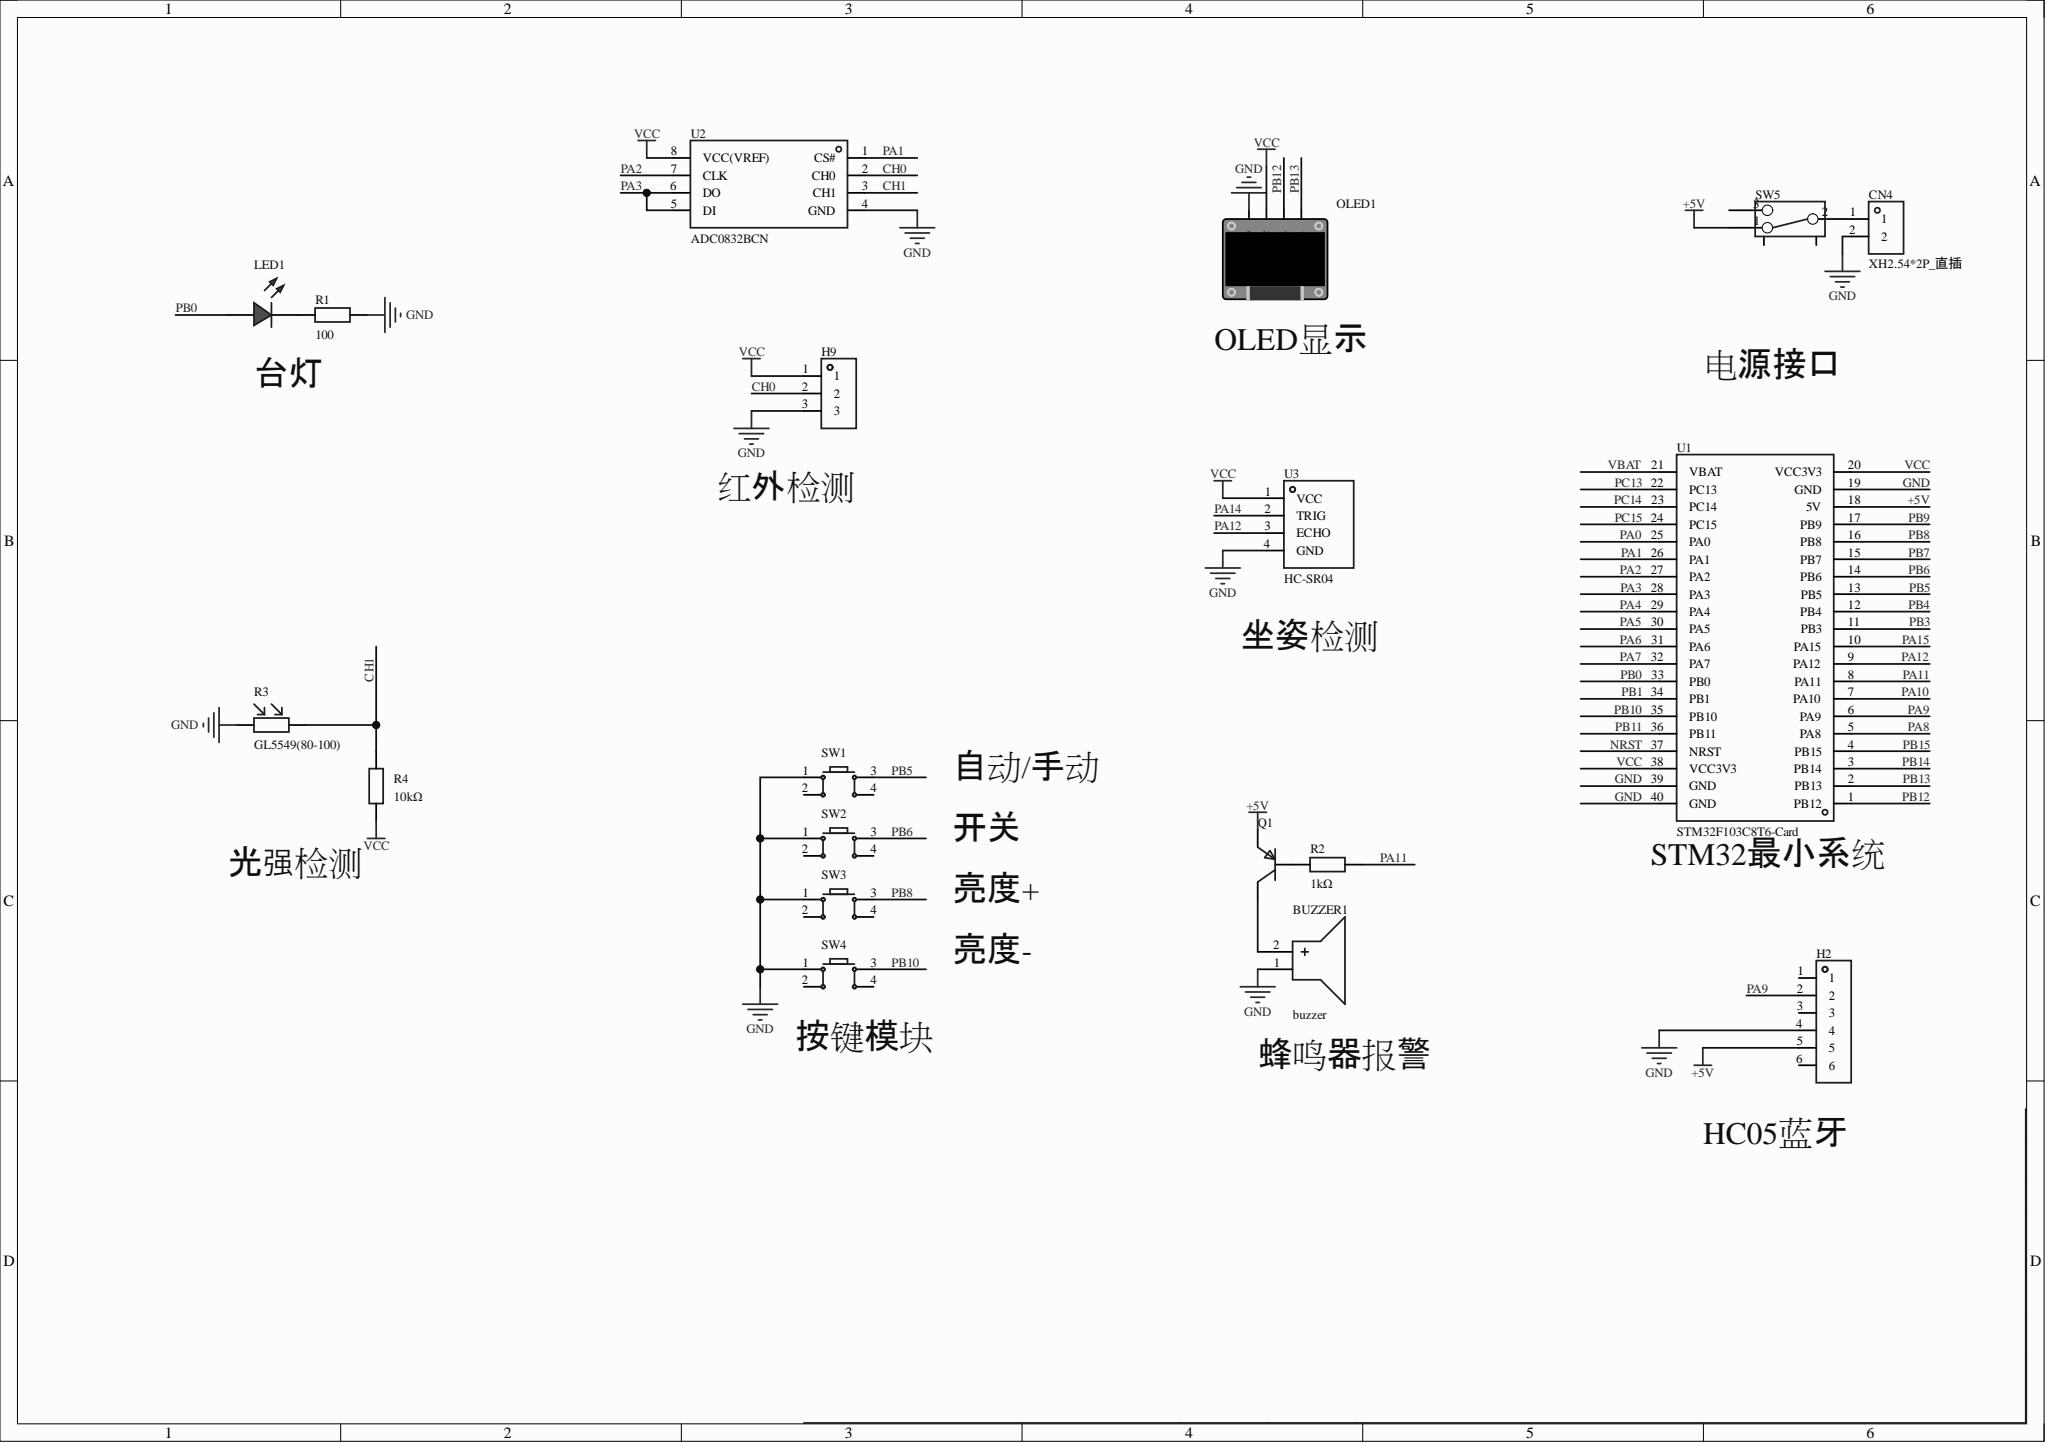Circuit board | Altium Designer | 19 parts | 22 nets
Bill of materials:
Comment,Description,Designator,Footprint,LibRef,Quantity
"buzzer","","BUZZER1","BUZ-TH_BD12.0-P6.00-D0.9-RD","buzzer","1"
"XH2.54*2P_直插","","CN4","CONN-TH_2P-P2.50-XH2.54-2P","XH2.54*2P_直插","1"
"","","H2","HDR-TH_6P-P2.54-V-F","HDR-F_2.54_1x6P","1"
"","","H9","HDR-TH_3P-P2.54-V-F","HDR-F_2.54_1x3P","1"
"","","LED1","LED_TH-3mm","LED_TH-R_3mm","1"
"","","OLED1","0.96OLED_4P","0.96OLED模块_4P","1"
"","","Q1","S8550P_TO-92","S8550_TO_PNP","1"
"100","","R1","Res_1/8W","Res_AXIAL-1/8W","1"
"1kΩ","","R2","Res_1/8W","Res_AXIAL-1/8W","1"
"GL5549(80-100)","","R3","RES-TH_L5.1-W4.3-P3.40-D0.5","GL5549(80-100)","1"
"10kΩ","","R4","Res_1/8W","Res_AXIAL-1/8W","1"
"","","SW1, SW2, SW3, SW4","SW-TH_4P-L6.0-W6.0-P4.50-LS6.5","Key_TH_6x6x6","4"
"","","SW5","拨动开关","拨动开关_正","1"
"STM32F103C8T6-Card","","U1","CONN-TH_L53.3-W22.9_STM32F103C8T6-CARD","STM32F103C8T6-Card","1"
"ADC0832BCN","分辨率:8位;工作电压:4.5V~6.3V;","U2","PDIP-8_L9.6-W6.4-P2.54-LS7.6-BL","ADC0832BCN","1"
"HC-SR04","","U3","TH_HC-SR04V","HC-SR04","1"
Netlist (Protel format):
[
BUZZER1
BUZ-TH_BD12.0-P6.00-D0.9-RD
buzzer



]
[
CN4
CONN-TH_2P-P2.50-XH2.54-2P
XH2.54*2P_直插



]
[
H2
HDR-TH_6P-P2.54-V-F




]
[
H9
HDR-TH_3P-P2.54-V-F




]
[
LED1
LED_TH-3mm




]
[
OLED1
0.96OLED_4P




]
[
Q1
S8550P_TO-92




]
[
R1
Res_1/8W
100



]
[
R2
Res_1/8W
1kΩ



]
[
R3
RES-TH_L5.1-W4.3-P3.40-D0.5
GL5549(80-100)



]
[
R4
Res_1/8W
10kΩ



]
[
SW1
SW-TH_4P-L6.0-W6.0-P4.50-LS6.5




]
[
SW2
SW-TH_4P-L6.0-W6.0-P4.50-LS6.5




]
[
SW3
SW-TH_4P-L6.0-W6.0-P4.50-LS6.5




]
[
SW4
SW-TH_4P-L6.0-W6.0-P4.50-LS6.5




]
[
SW5
拨动开关




]
[
U1
CONN-TH_L53.3-W22.9_STM32F103C8T6-CARD
STM32F103C8T6-Card



]
[
U2
PDIP-8_L9.6-W6.4-P2.54-LS7.6-BL
ADC0832BCN



]
[
U3
TH_HC-SR04V
HC-SR04



]
(
VCC
H9-1
OLED1-2
R4-1
U1-20
U1-38
U2-8
U3-1
)
(
PB13
OLED1-4
U1-2
)
(
PB12
OLED1-3
U1-1
)
(
PB10
SW4-3
U1-35
)
(
PB8
SW3-3
U1-16
)
(
PB6
SW2-3
U1-14
)
(
PB5
SW1-3
U1-13
)
(
PB0
LED1-1
U1-33
)
(
PA12
U1-9
U3-3
)
(
PA11
R2-2
U1-8
)
(
PA9
H2-2
U1-6
)
(
PA3
U1-28
U2-5
U2-6
)
(
PA2
U1-27
U2-7
)
(
PA1
U1-26
U2-1
)
(
NetQ1_2
Q1-2
R2-1
)
(
NetLED1_2
LED1-2
R1-1
)
(
NetCN4_1
CN4-1
SW5-2
)
(
NetBUZZER1_2
BUZZER1-2
Q1-3
)
(
GND
BUZZER1-1
CN4-2
H2-4
H9-3
OLED1-1
R1-2
R3-1
SW1-1
SW2-1
SW3-1
SW4-1
U1-19
U1-39
U1-40
U2-4
U3-4
)
(
CH1
R3-2
R4-2
U2-3
)
(
CH0
H9-2
U2-2
)
(
+5V
H2-5
Q1-1
SW5-1
U1-18
)